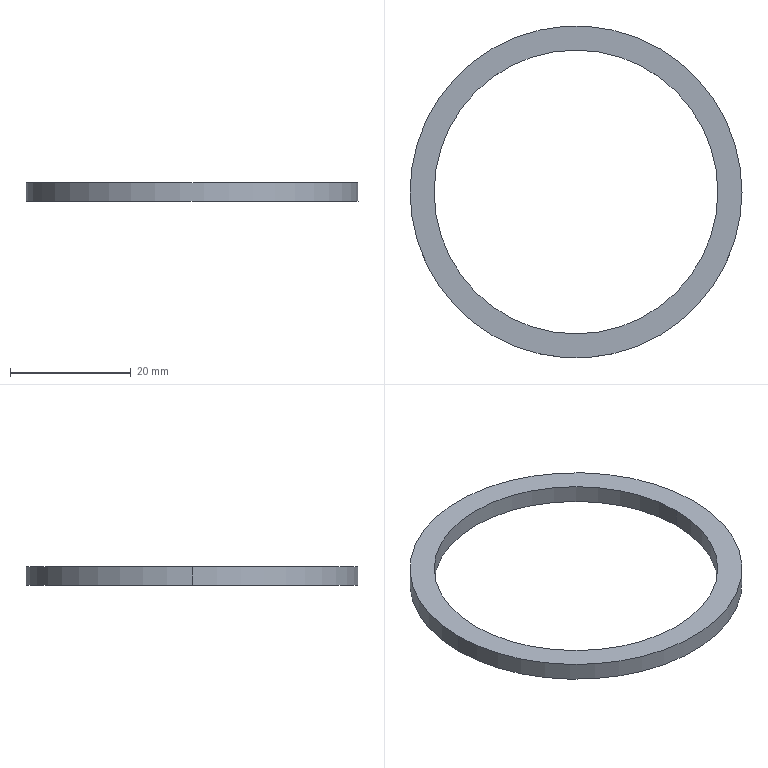Part | SolidWorks | features BaseBody 1 | 1 solid | 6 faces | box 55 x 55 x 3 mm | volume 1923 mm3 | cylinder 4 | plane 2 | commonest cylinder face diameters 47 x2 55 x2
STEP:
#1=CARTESIAN_POINT('',(-23.5,0.,1.5));
#2=VERTEX_POINT('',#1);
#3=CARTESIAN_POINT('',(23.5,0.,1.5));
#4=VERTEX_POINT('',#3);
#5=CARTESIAN_POINT('',(0.,0.,1.5));
#6=DIRECTION('',(0.,0.,1.));
#7=DIRECTION('',(1.,0.,0.));
#8=AXIS2_PLACEMENT_3D('',#5,#6,#7);
#9=CIRCLE('',#8,23.5);
#10=EDGE_CURVE('',#2,#4,#9,.T.);
#11=ORIENTED_EDGE('',*,*,#10,.T.);
#12=CARTESIAN_POINT('',(23.5,0.,-1.5));
#13=VERTEX_POINT('',#12);
#14=CARTESIAN_POINT('',(23.5,0.,1.5));
#15=DIRECTION('',(0.,0.,-1.));
#16=VECTOR('',#15,1000.);
#17=LINE('',#14,#16);
#18=EDGE_CURVE('',#4,#13,#17,.T.);
#19=ORIENTED_EDGE('',*,*,#18,.T.);
#20=CARTESIAN_POINT('',(-23.5,0.,-1.5));
#21=VERTEX_POINT('',#20);
#22=CARTESIAN_POINT('',(0.,0.,-1.5));
#23=DIRECTION('',(0.,0.,1.));
#24=DIRECTION('',(1.,0.,0.));
#25=AXIS2_PLACEMENT_3D('',#22,#23,#24);
#26=CIRCLE('',#25,23.5);
#27=EDGE_CURVE('',#21,#13,#26,.T.);
#28=ORIENTED_EDGE('',*,*,#27,.F.);
#29=CARTESIAN_POINT('',(-23.5,0.,1.5));
#30=DIRECTION('',(0.,0.,-1.));
#31=VECTOR('',#30,1000.);
#32=LINE('',#29,#31);
#33=EDGE_CURVE('',#2,#21,#32,.T.);
#34=ORIENTED_EDGE('',*,*,#33,.F.);
#35=EDGE_LOOP('',(#11,#19,#28,#34));
#36=FACE_OUTER_BOUND('',#35,.T.);
#37=CARTESIAN_POINT('',(0.,0.,1.5));
#38=DIRECTION('',(0.,0.,-1.));
#39=DIRECTION('',(-1.,0.,0.));
#40=AXIS2_PLACEMENT_3D('',#37,#38,#39);
#41=CYLINDRICAL_SURFACE('',#40,23.5);
#42=ADVANCED_FACE('',(#36),#41,.F.);
#43=CARTESIAN_POINT('',(27.5,0.,1.5));
#44=VERTEX_POINT('',#43);
#45=CARTESIAN_POINT('',(-27.5,0.,1.5));
#46=VERTEX_POINT('',#45);
#47=CARTESIAN_POINT('',(0.,0.,1.5));
#48=DIRECTION('',(0.,0.,1.));
#49=DIRECTION('',(1.,0.,0.));
#50=AXIS2_PLACEMENT_3D('',#47,#48,#49);
#51=CIRCLE('',#50,27.5);
#52=EDGE_CURVE('',#44,#46,#51,.T.);
#53=ORIENTED_EDGE('',*,*,#52,.F.);
#54=CARTESIAN_POINT('',(27.5,0.,-1.5));
#55=VERTEX_POINT('',#54);
#56=CARTESIAN_POINT('',(27.5,0.,1.5));
#57=DIRECTION('',(0.,0.,-1.));
#58=VECTOR('',#57,1000.);
#59=LINE('',#56,#58);
#60=EDGE_CURVE('',#44,#55,#59,.T.);
#61=ORIENTED_EDGE('',*,*,#60,.T.);
#62=CARTESIAN_POINT('',(-27.5,0.,-1.5));
#63=VERTEX_POINT('',#62);
#64=CARTESIAN_POINT('',(0.,0.,-1.5));
#65=DIRECTION('',(0.,0.,1.));
#66=DIRECTION('',(1.,0.,0.));
#67=AXIS2_PLACEMENT_3D('',#64,#65,#66);
#68=CIRCLE('',#67,27.5);
#69=EDGE_CURVE('',#55,#63,#68,.T.);
#70=ORIENTED_EDGE('',*,*,#69,.T.);
#71=CARTESIAN_POINT('',(-27.5,0.,1.5));
#72=DIRECTION('',(0.,0.,-1.));
#73=VECTOR('',#72,1000.);
#74=LINE('',#71,#73);
#75=EDGE_CURVE('',#46,#63,#74,.T.);
#76=ORIENTED_EDGE('',*,*,#75,.F.);
#77=EDGE_LOOP('',(#53,#61,#70,#76));
#78=FACE_OUTER_BOUND('',#77,.T.);
#79=CARTESIAN_POINT('',(0.,0.,1.5));
#80=DIRECTION('',(0.,0.,-1.));
#81=DIRECTION('',(-1.,0.,0.));
#82=AXIS2_PLACEMENT_3D('',#79,#80,#81);
#83=CYLINDRICAL_SURFACE('',#82,27.5);
#84=ADVANCED_FACE('',(#78),#83,.T.);
#85=ORIENTED_EDGE('',*,*,#27,.T.);
#86=CARTESIAN_POINT('',(0.,0.,-1.5));
#87=DIRECTION('',(0.,0.,1.));
#88=DIRECTION('',(1.,0.,0.));
#89=AXIS2_PLACEMENT_3D('',#86,#87,#88);
#90=CIRCLE('',#89,23.5);
#91=EDGE_CURVE('',#13,#21,#90,.T.);
#92=ORIENTED_EDGE('',*,*,#91,.T.);
#93=EDGE_LOOP('',(#85,#92));
#94=FACE_BOUND('',#93,.T.);
#95=CARTESIAN_POINT('',(0.,0.,-1.5));
#96=DIRECTION('',(0.,0.,1.));
#97=DIRECTION('',(1.,0.,0.));
#98=AXIS2_PLACEMENT_3D('',#95,#96,#97);
#99=CIRCLE('',#98,27.5);
#100=EDGE_CURVE('',#63,#55,#99,.T.);
#101=ORIENTED_EDGE('',*,*,#100,.F.);
#102=ORIENTED_EDGE('',*,*,#69,.F.);
#103=EDGE_LOOP('',(#101,#102));
#104=FACE_OUTER_BOUND('',#103,.T.);
#105=CARTESIAN_POINT('',(0.,0.,-1.5));
#106=DIRECTION('',(0.,0.,1.));
#107=DIRECTION('',(1.,0.,0.));
#108=AXIS2_PLACEMENT_3D('',#105,#106,#107);
#109=PLANE('',#108);
#110=ADVANCED_FACE('',(#94,#104),#109,.F.);
#111=ORIENTED_EDGE('',*,*,#10,.F.);
#112=CARTESIAN_POINT('',(0.,0.,1.5));
#113=DIRECTION('',(0.,0.,1.));
#114=DIRECTION('',(1.,0.,0.));
#115=AXIS2_PLACEMENT_3D('',#112,#113,#114);
#116=CIRCLE('',#115,23.5);
#117=EDGE_CURVE('',#4,#2,#116,.T.);
#118=ORIENTED_EDGE('',*,*,#117,.F.);
#119=EDGE_LOOP('',(#111,#118));
#120=FACE_BOUND('',#119,.T.);
#121=CARTESIAN_POINT('',(0.,0.,1.5));
#122=DIRECTION('',(0.,0.,1.));
#123=DIRECTION('',(1.,0.,0.));
#124=AXIS2_PLACEMENT_3D('',#121,#122,#123);
#125=CIRCLE('',#124,27.5);
#126=EDGE_CURVE('',#46,#44,#125,.T.);
#127=ORIENTED_EDGE('',*,*,#126,.T.);
#128=ORIENTED_EDGE('',*,*,#52,.T.);
#129=EDGE_LOOP('',(#127,#128));
#130=FACE_OUTER_BOUND('',#129,.T.);
#131=CARTESIAN_POINT('',(0.,0.,1.5));
#132=DIRECTION('',(0.,0.,1.));
#133=DIRECTION('',(1.,0.,0.));
#134=AXIS2_PLACEMENT_3D('',#131,#132,#133);
#135=PLANE('',#134);
#136=ADVANCED_FACE('',(#120,#130),#135,.T.);
#137=ORIENTED_EDGE('',*,*,#60,.F.);
#138=ORIENTED_EDGE('',*,*,#126,.F.);
#139=ORIENTED_EDGE('',*,*,#75,.T.);
#140=ORIENTED_EDGE('',*,*,#100,.T.);
#141=EDGE_LOOP('',(#137,#138,#139,#140));
#142=FACE_OUTER_BOUND('',#141,.T.);
#143=CARTESIAN_POINT('',(0.,0.,1.5));
#144=DIRECTION('',(0.,0.,-1.));
#145=DIRECTION('',(-1.,0.,0.));
#146=AXIS2_PLACEMENT_3D('',#143,#144,#145);
#147=CYLINDRICAL_SURFACE('',#146,27.5);
#148=ADVANCED_FACE('',(#142),#147,.T.);
#149=ORIENTED_EDGE('',*,*,#18,.F.);
#150=ORIENTED_EDGE('',*,*,#117,.T.);
#151=ORIENTED_EDGE('',*,*,#33,.T.);
#152=ORIENTED_EDGE('',*,*,#91,.F.);
#153=EDGE_LOOP('',(#149,#150,#151,#152));
#154=FACE_OUTER_BOUND('',#153,.T.);
#155=CARTESIAN_POINT('',(0.,0.,1.5));
#156=DIRECTION('',(0.,0.,-1.));
#157=DIRECTION('',(-1.,0.,0.));
#158=AXIS2_PLACEMENT_3D('',#155,#156,#157);
#159=CYLINDRICAL_SURFACE('',#158,23.5);
#160=ADVANCED_FACE('',(#154),#159,.F.);
#161=CLOSED_SHELL('',(#42,#84,#110,#136,#148,#160));
#162=MANIFOLD_SOLID_BREP('',#161);
#163=CARTESIAN_POINT('',(0.,0.,0.));
#164=DIRECTION('',(0.,0.,1.));
#165=DIRECTION('',(1.,0.,0.));
#166=AXIS2_PLACEMENT_3D('',#163,#164,#165);
#167=(LENGTH_UNIT()NAMED_UNIT(*)SI_UNIT(.MILLI.,.METRE.));
#168=UNCERTAINTY_MEASURE_WITH_UNIT(LENGTH_MEASURE(0.00001),#167,'','');
#169=(NAMED_UNIT(*)PLANE_ANGLE_UNIT()SI_UNIT($,.RADIAN.));
#170=(NAMED_UNIT(*)SI_UNIT($,.STERADIAN.)SOLID_ANGLE_UNIT());
#171=(GEOMETRIC_REPRESENTATION_CONTEXT(3)GLOBAL_UNCERTAINTY_ASSIGNED_CONTEXT((#168))GLOBAL_UNIT_ASSIGNED_CONTEXT((#167,#169,#170))REPRESENTATION_CONTEXT('',''));
#172=ADVANCED_BREP_SHAPE_REPRESENTATION('',(#162,#166),#171);